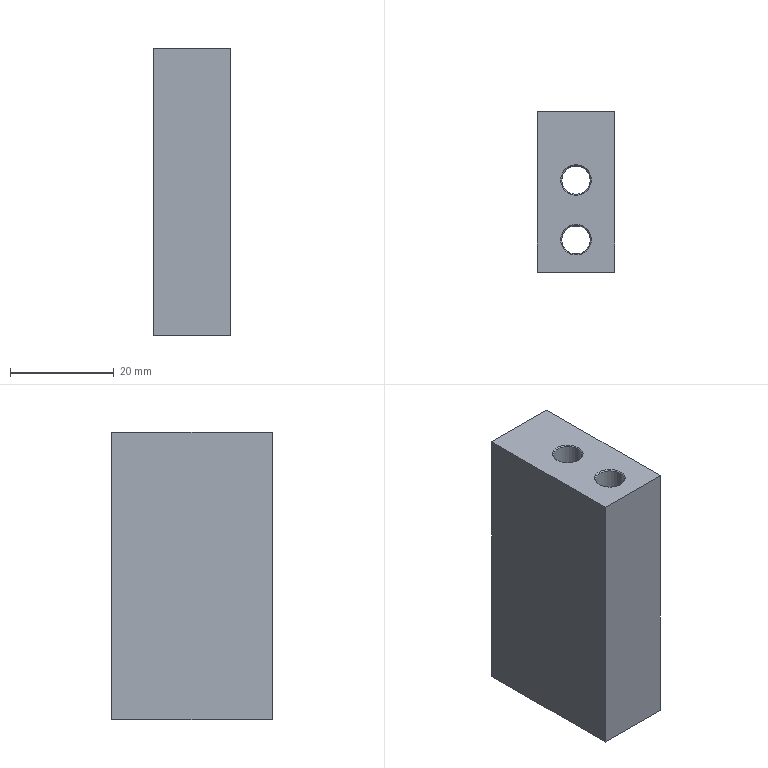Part | NX | 1 solid | 18 faces | box 15 x 31 x 55.4 mm | volume 23127 mm3 | cone 8 | plane 6 | cylinder 4 | commonest cylinder face diameters 5.5 x4
STEP:
#1=CARTESIAN_POINT('',(-70.,176.7,-18.2));
#2=VERTEX_POINT('',#1);
#3=CARTESIAN_POINT('',(-70.,207.7,-18.2));
#4=VERTEX_POINT('',#3);
#5=CARTESIAN_POINT('',(-70.,194.022,-18.2));
#6=DIRECTION('',(0.,1.,0.));
#7=VECTOR('',#6,1000.);
#8=LINE('',#5,#7);
#9=EDGE_CURVE('',#2,#4,#8,.T.);
#10=ORIENTED_EDGE('',*,*,#9,.F.);
#11=CARTESIAN_POINT('',(-70.,176.7,37.2));
#12=VERTEX_POINT('',#11);
#13=CARTESIAN_POINT('',(-70.,176.7,-18.2));
#14=DIRECTION('',(0.,0.,1.));
#15=VECTOR('',#14,1000.);
#16=LINE('',#13,#15);
#17=EDGE_CURVE('',#2,#12,#16,.T.);
#18=ORIENTED_EDGE('',*,*,#17,.T.);
#19=CARTESIAN_POINT('',(-70.,207.7,37.2));
#20=VERTEX_POINT('',#19);
#21=CARTESIAN_POINT('',(-70.,194.022,37.2));
#22=DIRECTION('',(0.,1.,0.));
#23=VECTOR('',#22,1000.);
#24=LINE('',#21,#23);
#25=EDGE_CURVE('',#12,#20,#24,.T.);
#26=ORIENTED_EDGE('',*,*,#25,.T.);
#27=CARTESIAN_POINT('',(-70.,207.7,-18.2));
#28=DIRECTION('',(0.,0.,-1.));
#29=VECTOR('',#28,1000.);
#30=LINE('',#27,#29);
#31=EDGE_CURVE('',#20,#4,#30,.T.);
#32=ORIENTED_EDGE('',*,*,#31,.T.);
#33=EDGE_LOOP('',(#10,#18,#26,#32));
#34=FACE_BOUND('',#33,.T.);
#35=CARTESIAN_POINT('',(-70.,169.7,-18.2));
#36=DIRECTION('',(-1.,0.,0.));
#37=DIRECTION('',(0.,0.,1.));
#38=AXIS2_PLACEMENT_3D('',#35,#36,#37);
#39=PLANE('',#38);
#40=ADVANCED_FACE('',(#34),#39,.T.);
#41=CARTESIAN_POINT('',(-55.,176.7,-18.2));
#42=VERTEX_POINT('',#41);
#43=CARTESIAN_POINT('',(-61.534,176.7,-18.2));
#44=DIRECTION('',(1.,0.,0.));
#45=VECTOR('',#44,1000.);
#46=LINE('',#43,#45);
#47=EDGE_CURVE('',#2,#42,#46,.T.);
#48=ORIENTED_EDGE('',*,*,#47,.T.);
#49=CARTESIAN_POINT('',(-55.,176.7,37.2));
#50=VERTEX_POINT('',#49);
#51=CARTESIAN_POINT('',(-55.,176.7,-18.2));
#52=DIRECTION('',(0.,0.,-1.));
#53=VECTOR('',#52,1000.);
#54=LINE('',#51,#53);
#55=EDGE_CURVE('',#50,#42,#54,.T.);
#56=ORIENTED_EDGE('',*,*,#55,.F.);
#57=CARTESIAN_POINT('',(-61.534,176.7,37.2));
#58=DIRECTION('',(1.,0.,0.));
#59=VECTOR('',#58,1000.);
#60=LINE('',#57,#59);
#61=EDGE_CURVE('',#12,#50,#60,.T.);
#62=ORIENTED_EDGE('',*,*,#61,.F.);
#63=ORIENTED_EDGE('',*,*,#17,.F.);
#64=EDGE_LOOP('',(#48,#56,#62,#63));
#65=FACE_BOUND('',#64,.T.);
#66=CARTESIAN_POINT('',(-55.,176.7,-18.2));
#67=DIRECTION('',(0.,-1.,0.));
#68=DIRECTION('',(0.,0.,-1.));
#69=AXIS2_PLACEMENT_3D('',#66,#67,#68);
#70=PLANE('',#69);
#71=ADVANCED_FACE('',(#65),#70,.T.);
#72=CARTESIAN_POINT('',(-55.,207.7,-18.2));
#73=VERTEX_POINT('',#72);
#74=CARTESIAN_POINT('',(-55.,194.022,-18.2));
#75=DIRECTION('',(0.,-1.,0.));
#76=VECTOR('',#75,1000.);
#77=LINE('',#74,#76);
#78=EDGE_CURVE('',#73,#42,#77,.T.);
#79=ORIENTED_EDGE('',*,*,#78,.F.);
#80=CARTESIAN_POINT('',(-55.,207.7,37.2));
#81=VERTEX_POINT('',#80);
#82=CARTESIAN_POINT('',(-55.,207.7,-18.2));
#83=DIRECTION('',(0.,0.,1.));
#84=VECTOR('',#83,1000.);
#85=LINE('',#82,#84);
#86=EDGE_CURVE('',#73,#81,#85,.T.);
#87=ORIENTED_EDGE('',*,*,#86,.T.);
#88=CARTESIAN_POINT('',(-55.,194.022,37.2));
#89=DIRECTION('',(0.,-1.,0.));
#90=VECTOR('',#89,1000.);
#91=LINE('',#88,#90);
#92=EDGE_CURVE('',#81,#50,#91,.T.);
#93=ORIENTED_EDGE('',*,*,#92,.T.);
#94=ORIENTED_EDGE('',*,*,#55,.T.);
#95=EDGE_LOOP('',(#79,#87,#93,#94));
#96=FACE_BOUND('',#95,.T.);
#97=CARTESIAN_POINT('',(-55.,208.7,-18.2));
#98=DIRECTION('',(1.,0.,0.));
#99=DIRECTION('',(0.,1.,0.));
#100=AXIS2_PLACEMENT_3D('',#97,#98,#99);
#101=PLANE('',#100);
#102=ADVANCED_FACE('',(#96),#101,.T.);
#103=CARTESIAN_POINT('',(-61.534,207.7,-18.2));
#104=DIRECTION('',(-1.,0.,0.));
#105=VECTOR('',#104,1000.);
#106=LINE('',#103,#105);
#107=EDGE_CURVE('',#73,#4,#106,.T.);
#108=ORIENTED_EDGE('',*,*,#107,.T.);
#109=ORIENTED_EDGE('',*,*,#31,.F.);
#110=CARTESIAN_POINT('',(-61.534,207.7,37.2));
#111=DIRECTION('',(-1.,0.,0.));
#112=VECTOR('',#111,1000.);
#113=LINE('',#110,#112);
#114=EDGE_CURVE('',#81,#20,#113,.T.);
#115=ORIENTED_EDGE('',*,*,#114,.F.);
#116=ORIENTED_EDGE('',*,*,#86,.F.);
#117=EDGE_LOOP('',(#108,#109,#115,#116));
#118=FACE_BOUND('',#117,.T.);
#119=CARTESIAN_POINT('',(-70.,207.7,-18.2));
#120=DIRECTION('',(0.,1.,0.));
#121=DIRECTION('',(1.,0.,0.));
#122=AXIS2_PLACEMENT_3D('',#119,#120,#121);
#123=PLANE('',#122);
#124=ADVANCED_FACE('',(#118),#123,.T.);
#125=CARTESIAN_POINT('',(-65.25,194.45,37.));
#126=VERTEX_POINT('',#125);
#127=CARTESIAN_POINT('',(-59.75,194.45,37.));
#128=VERTEX_POINT('',#127);
#129=CARTESIAN_POINT('',(-62.5,194.45,37.));
#130=DIRECTION('',(0.,0.,1.));
#131=DIRECTION('',(1.,0.,0.));
#132=AXIS2_PLACEMENT_3D('',#129,#130,#131);
#133=CIRCLE('',#132,2.75);
#134=EDGE_CURVE('',#126,#128,#133,.T.);
#135=ORIENTED_EDGE('',*,*,#134,.T.);
#136=CARTESIAN_POINT('',(-59.75,194.45,-18.));
#137=VERTEX_POINT('',#136);
#138=CARTESIAN_POINT('',(-59.75,194.45,37.2));
#139=DIRECTION('',(0.,0.,1.));
#140=VECTOR('',#139,1000.);
#141=LINE('',#138,#140);
#142=EDGE_CURVE('',#137,#128,#141,.T.);
#143=ORIENTED_EDGE('',*,*,#142,.F.);
#144=CARTESIAN_POINT('',(-65.25,194.45,-18.));
#145=VERTEX_POINT('',#144);
#146=CARTESIAN_POINT('',(-62.5,194.45,-18.));
#147=DIRECTION('',(0.,0.,1.));
#148=DIRECTION('',(1.,0.,0.));
#149=AXIS2_PLACEMENT_3D('',#146,#147,#148);
#150=CIRCLE('',#149,2.75);
#151=EDGE_CURVE('',#145,#137,#150,.T.);
#152=ORIENTED_EDGE('',*,*,#151,.F.);
#153=CARTESIAN_POINT('',(-65.25,194.45,37.2));
#154=DIRECTION('',(0.,0.,1.));
#155=VECTOR('',#154,1000.);
#156=LINE('',#153,#155);
#157=EDGE_CURVE('',#145,#126,#156,.T.);
#158=ORIENTED_EDGE('',*,*,#157,.T.);
#159=EDGE_LOOP('',(#135,#143,#152,#158));
#160=FACE_BOUND('',#159,.T.);
#161=CARTESIAN_POINT('',(-62.5,194.45,37.2));
#162=DIRECTION('',(0.,0.,1.));
#163=DIRECTION('',(1.,0.,0.));
#164=AXIS2_PLACEMENT_3D('',#161,#162,#163);
#165=CYLINDRICAL_SURFACE('',#164,2.75);
#166=ADVANCED_FACE('',(#160),#165,.F.);
#167=CARTESIAN_POINT('',(-65.45,194.45,37.2));
#168=VERTEX_POINT('',#167);
#169=CARTESIAN_POINT('',(-59.55,194.45,37.2));
#170=VERTEX_POINT('',#169);
#171=CARTESIAN_POINT('',(-62.5,194.45,37.2));
#172=DIRECTION('',(0.,0.,1.));
#173=DIRECTION('',(1.,0.,0.));
#174=AXIS2_PLACEMENT_3D('',#171,#172,#173);
#175=CIRCLE('',#174,2.95);
#176=EDGE_CURVE('',#168,#170,#175,.T.);
#177=ORIENTED_EDGE('',*,*,#176,.T.);
#178=CARTESIAN_POINT('',(-59.75,194.45,37.));
#179=DIRECTION('',(0.7071,0.,0.7071));
#180=VECTOR('',#179,1000.);
#181=LINE('',#178,#180);
#182=EDGE_CURVE('',#128,#170,#181,.T.);
#183=ORIENTED_EDGE('',*,*,#182,.F.);
#184=ORIENTED_EDGE('',*,*,#134,.F.);
#185=CARTESIAN_POINT('',(-65.25,194.45,37.));
#186=DIRECTION('',(-0.7071,0.,0.7071));
#187=VECTOR('',#186,1000.);
#188=LINE('',#185,#187);
#189=EDGE_CURVE('',#126,#168,#188,.T.);
#190=ORIENTED_EDGE('',*,*,#189,.T.);
#191=EDGE_LOOP('',(#177,#183,#184,#190));
#192=FACE_BOUND('',#191,.T.);
#193=CARTESIAN_POINT('',(-62.5,194.45,37.));
#194=DIRECTION('',(0.,0.,1.));
#195=DIRECTION('',(1.,0.,0.));
#196=AXIS2_PLACEMENT_3D('',#193,#194,#195);
#197=CONICAL_SURFACE('',#196,2.75,0.7854);
#198=ADVANCED_FACE('',(#192),#197,.F.);
#199=ORIENTED_EDGE('',*,*,#151,.T.);
#200=CARTESIAN_POINT('',(-59.55,194.45,-18.2));
#201=VERTEX_POINT('',#200);
#202=CARTESIAN_POINT('',(-59.75,194.45,-18.));
#203=DIRECTION('',(0.7071,0.,-0.7071));
#204=VECTOR('',#203,1000.);
#205=LINE('',#202,#204);
#206=EDGE_CURVE('',#201,#137,#205,.F.);
#207=ORIENTED_EDGE('',*,*,#206,.F.);
#208=CARTESIAN_POINT('',(-65.45,194.45,-18.2));
#209=VERTEX_POINT('',#208);
#210=CARTESIAN_POINT('',(-62.5,194.45,-18.2));
#211=DIRECTION('',(0.,0.,1.));
#212=DIRECTION('',(1.,0.,0.));
#213=AXIS2_PLACEMENT_3D('',#210,#211,#212);
#214=CIRCLE('',#213,2.95);
#215=EDGE_CURVE('',#209,#201,#214,.T.);
#216=ORIENTED_EDGE('',*,*,#215,.F.);
#217=CARTESIAN_POINT('',(-65.25,194.45,-18.));
#218=DIRECTION('',(-0.7071,0.,-0.7071));
#219=VECTOR('',#218,1000.);
#220=LINE('',#217,#219);
#221=EDGE_CURVE('',#209,#145,#220,.F.);
#222=ORIENTED_EDGE('',*,*,#221,.T.);
#223=EDGE_LOOP('',(#199,#207,#216,#222));
#224=FACE_BOUND('',#223,.T.);
#225=CARTESIAN_POINT('',(-62.5,194.45,-18.));
#226=DIRECTION('',(0.,0.,-1.));
#227=DIRECTION('',(-1.,0.,0.));
#228=AXIS2_PLACEMENT_3D('',#225,#226,#227);
#229=CONICAL_SURFACE('',#228,2.75,0.7854);
#230=ADVANCED_FACE('',(#224),#229,.F.);
#231=CARTESIAN_POINT('',(-59.75,182.95,-18.));
#232=VERTEX_POINT('',#231);
#233=CARTESIAN_POINT('',(-65.25,182.95,-18.));
#234=VERTEX_POINT('',#233);
#235=CARTESIAN_POINT('',(-62.5,182.95,-18.));
#236=DIRECTION('',(0.,0.,1.));
#237=DIRECTION('',(1.,0.,0.));
#238=AXIS2_PLACEMENT_3D('',#235,#236,#237);
#239=CIRCLE('',#238,2.75);
#240=EDGE_CURVE('',#232,#234,#239,.T.);
#241=ORIENTED_EDGE('',*,*,#240,.T.);
#242=CARTESIAN_POINT('',(-65.45,182.95,-18.2));
#243=VERTEX_POINT('',#242);
#244=CARTESIAN_POINT('',(-65.25,182.95,-18.));
#245=DIRECTION('',(-0.7071,0.,-0.7071));
#246=VECTOR('',#245,1000.);
#247=LINE('',#244,#246);
#248=EDGE_CURVE('',#243,#234,#247,.F.);
#249=ORIENTED_EDGE('',*,*,#248,.F.);
#250=CARTESIAN_POINT('',(-59.55,182.95,-18.2));
#251=VERTEX_POINT('',#250);
#252=CARTESIAN_POINT('',(-62.5,182.95,-18.2));
#253=DIRECTION('',(0.,0.,1.));
#254=DIRECTION('',(1.,0.,0.));
#255=AXIS2_PLACEMENT_3D('',#252,#253,#254);
#256=CIRCLE('',#255,2.95);
#257=EDGE_CURVE('',#251,#243,#256,.T.);
#258=ORIENTED_EDGE('',*,*,#257,.F.);
#259=CARTESIAN_POINT('',(-59.75,182.95,-18.));
#260=DIRECTION('',(0.7071,0.,-0.7071));
#261=VECTOR('',#260,1000.);
#262=LINE('',#259,#261);
#263=EDGE_CURVE('',#251,#232,#262,.F.);
#264=ORIENTED_EDGE('',*,*,#263,.T.);
#265=EDGE_LOOP('',(#241,#249,#258,#264));
#266=FACE_BOUND('',#265,.T.);
#267=CARTESIAN_POINT('',(-62.5,182.95,-18.));
#268=DIRECTION('',(0.,0.,-1.));
#269=DIRECTION('',(-1.,0.,0.));
#270=AXIS2_PLACEMENT_3D('',#267,#268,#269);
#271=CONICAL_SURFACE('',#270,2.75,0.7854);
#272=ADVANCED_FACE('',(#266),#271,.F.);
#273=CARTESIAN_POINT('',(-65.25,182.95,37.));
#274=VERTEX_POINT('',#273);
#275=CARTESIAN_POINT('',(-59.75,182.95,37.));
#276=VERTEX_POINT('',#275);
#277=CARTESIAN_POINT('',(-62.5,182.95,37.));
#278=DIRECTION('',(0.,0.,1.));
#279=DIRECTION('',(1.,0.,0.));
#280=AXIS2_PLACEMENT_3D('',#277,#278,#279);
#281=CIRCLE('',#280,2.75);
#282=EDGE_CURVE('',#274,#276,#281,.T.);
#283=ORIENTED_EDGE('',*,*,#282,.F.);
#284=CARTESIAN_POINT('',(-65.45,182.95,37.2));
#285=VERTEX_POINT('',#284);
#286=CARTESIAN_POINT('',(-65.25,182.95,37.));
#287=DIRECTION('',(-0.7071,0.,0.7071));
#288=VECTOR('',#287,1000.);
#289=LINE('',#286,#288);
#290=EDGE_CURVE('',#285,#274,#289,.F.);
#291=ORIENTED_EDGE('',*,*,#290,.F.);
#292=CARTESIAN_POINT('',(-59.55,182.95,37.2));
#293=VERTEX_POINT('',#292);
#294=CARTESIAN_POINT('',(-62.5,182.95,37.2));
#295=DIRECTION('',(0.,0.,1.));
#296=DIRECTION('',(1.,0.,0.));
#297=AXIS2_PLACEMENT_3D('',#294,#295,#296);
#298=CIRCLE('',#297,2.95);
#299=EDGE_CURVE('',#285,#293,#298,.T.);
#300=ORIENTED_EDGE('',*,*,#299,.T.);
#301=CARTESIAN_POINT('',(-59.75,182.95,37.));
#302=DIRECTION('',(0.7071,0.,0.7071));
#303=VECTOR('',#302,1000.);
#304=LINE('',#301,#303);
#305=EDGE_CURVE('',#293,#276,#304,.F.);
#306=ORIENTED_EDGE('',*,*,#305,.T.);
#307=EDGE_LOOP('',(#283,#291,#300,#306));
#308=FACE_BOUND('',#307,.T.);
#309=CARTESIAN_POINT('',(-62.5,182.95,37.));
#310=DIRECTION('',(0.,0.,1.));
#311=DIRECTION('',(1.,0.,0.));
#312=AXIS2_PLACEMENT_3D('',#309,#310,#311);
#313=CONICAL_SURFACE('',#312,2.75,0.7854);
#314=ADVANCED_FACE('',(#308),#313,.F.);
#315=ORIENTED_EDGE('',*,*,#47,.F.);
#316=ORIENTED_EDGE('',*,*,#9,.T.);
#317=ORIENTED_EDGE('',*,*,#107,.F.);
#318=ORIENTED_EDGE('',*,*,#78,.T.);
#319=EDGE_LOOP('',(#315,#316,#317,#318));
#320=FACE_BOUND('',#319,.T.);
#321=ORIENTED_EDGE('',*,*,#215,.T.);
#322=CARTESIAN_POINT('',(-62.5,194.45,-18.2));
#323=DIRECTION('',(0.,0.,1.));
#324=DIRECTION('',(1.,0.,0.));
#325=AXIS2_PLACEMENT_3D('',#322,#323,#324);
#326=CIRCLE('',#325,2.95);
#327=EDGE_CURVE('',#201,#209,#326,.T.);
#328=ORIENTED_EDGE('',*,*,#327,.T.);
#329=EDGE_LOOP('',(#321,#328));
#330=FACE_BOUND('',#329,.T.);
#331=CARTESIAN_POINT('',(-62.5,182.95,-18.2));
#332=DIRECTION('',(0.,0.,1.));
#333=DIRECTION('',(1.,0.,0.));
#334=AXIS2_PLACEMENT_3D('',#331,#332,#333);
#335=CIRCLE('',#334,2.95);
#336=EDGE_CURVE('',#243,#251,#335,.T.);
#337=ORIENTED_EDGE('',*,*,#336,.T.);
#338=ORIENTED_EDGE('',*,*,#257,.T.);
#339=EDGE_LOOP('',(#337,#338));
#340=FACE_BOUND('',#339,.T.);
#341=CARTESIAN_POINT('',(-61.534,194.022,-18.2));
#342=DIRECTION('',(0.,0.,1.));
#343=DIRECTION('',(1.,0.,0.));
#344=AXIS2_PLACEMENT_3D('',#341,#342,#343);
#345=PLANE('',#344);
#346=ADVANCED_FACE('',(#320,#330,#340),#345,.F.);
#347=ORIENTED_EDGE('',*,*,#92,.F.);
#348=ORIENTED_EDGE('',*,*,#114,.T.);
#349=ORIENTED_EDGE('',*,*,#25,.F.);
#350=ORIENTED_EDGE('',*,*,#61,.T.);
#351=EDGE_LOOP('',(#347,#348,#349,#350));
#352=FACE_BOUND('',#351,.T.);
#353=ORIENTED_EDGE('',*,*,#176,.F.);
#354=CARTESIAN_POINT('',(-62.5,194.45,37.2));
#355=DIRECTION('',(0.,0.,1.));
#356=DIRECTION('',(1.,0.,0.));
#357=AXIS2_PLACEMENT_3D('',#354,#355,#356);
#358=CIRCLE('',#357,2.95);
#359=EDGE_CURVE('',#170,#168,#358,.T.);
#360=ORIENTED_EDGE('',*,*,#359,.F.);
#361=EDGE_LOOP('',(#353,#360));
#362=FACE_BOUND('',#361,.T.);
#363=CARTESIAN_POINT('',(-62.5,182.95,37.2));
#364=DIRECTION('',(0.,0.,1.));
#365=DIRECTION('',(1.,0.,0.));
#366=AXIS2_PLACEMENT_3D('',#363,#364,#365);
#367=CIRCLE('',#366,2.95);
#368=EDGE_CURVE('',#293,#285,#367,.T.);
#369=ORIENTED_EDGE('',*,*,#368,.F.);
#370=ORIENTED_EDGE('',*,*,#299,.F.);
#371=EDGE_LOOP('',(#369,#370));
#372=FACE_BOUND('',#371,.T.);
#373=CARTESIAN_POINT('',(-61.534,194.022,37.2));
#374=DIRECTION('',(0.,0.,1.));
#375=DIRECTION('',(1.,0.,0.));
#376=AXIS2_PLACEMENT_3D('',#373,#374,#375);
#377=PLANE('',#376);
#378=ADVANCED_FACE('',(#352,#362,#372),#377,.T.);
#379=ORIENTED_EDGE('',*,*,#240,.F.);
#380=CARTESIAN_POINT('',(-59.75,182.95,37.2));
#381=DIRECTION('',(0.,0.,1.));
#382=VECTOR('',#381,1000.);
#383=LINE('',#380,#382);
#384=EDGE_CURVE('',#232,#276,#383,.T.);
#385=ORIENTED_EDGE('',*,*,#384,.T.);
#386=CARTESIAN_POINT('',(-62.5,182.95,37.));
#387=DIRECTION('',(0.,0.,1.));
#388=DIRECTION('',(1.,0.,0.));
#389=AXIS2_PLACEMENT_3D('',#386,#387,#388);
#390=CIRCLE('',#389,2.75);
#391=EDGE_CURVE('',#276,#274,#390,.T.);
#392=ORIENTED_EDGE('',*,*,#391,.T.);
#393=CARTESIAN_POINT('',(-65.25,182.95,37.2));
#394=DIRECTION('',(0.,0.,1.));
#395=VECTOR('',#394,1000.);
#396=LINE('',#393,#395);
#397=EDGE_CURVE('',#234,#274,#396,.T.);
#398=ORIENTED_EDGE('',*,*,#397,.F.);
#399=EDGE_LOOP('',(#379,#385,#392,#398));
#400=FACE_BOUND('',#399,.T.);
#401=CARTESIAN_POINT('',(-62.5,182.95,37.2));
#402=DIRECTION('',(0.,0.,1.));
#403=DIRECTION('',(1.,0.,0.));
#404=AXIS2_PLACEMENT_3D('',#401,#402,#403);
#405=CYLINDRICAL_SURFACE('',#404,2.75);
#406=ADVANCED_FACE('',(#400),#405,.F.);
#407=ORIENTED_EDGE('',*,*,#368,.T.);
#408=ORIENTED_EDGE('',*,*,#290,.T.);
#409=ORIENTED_EDGE('',*,*,#391,.F.);
#410=ORIENTED_EDGE('',*,*,#305,.F.);
#411=EDGE_LOOP('',(#407,#408,#409,#410));
#412=FACE_BOUND('',#411,.T.);
#413=CARTESIAN_POINT('',(-62.5,182.95,37.));
#414=DIRECTION('',(0.,0.,1.));
#415=DIRECTION('',(1.,0.,0.));
#416=AXIS2_PLACEMENT_3D('',#413,#414,#415);
#417=CONICAL_SURFACE('',#416,2.75,0.7854);
#418=ADVANCED_FACE('',(#412),#417,.F.);
#419=ORIENTED_EDGE('',*,*,#182,.T.);
#420=ORIENTED_EDGE('',*,*,#359,.T.);
#421=ORIENTED_EDGE('',*,*,#189,.F.);
#422=CARTESIAN_POINT('',(-62.5,194.45,37.));
#423=DIRECTION('',(0.,0.,1.));
#424=DIRECTION('',(1.,0.,0.));
#425=AXIS2_PLACEMENT_3D('',#422,#423,#424);
#426=CIRCLE('',#425,2.75);
#427=EDGE_CURVE('',#128,#126,#426,.T.);
#428=ORIENTED_EDGE('',*,*,#427,.F.);
#429=EDGE_LOOP('',(#419,#420,#421,#428));
#430=FACE_BOUND('',#429,.T.);
#431=CARTESIAN_POINT('',(-62.5,194.45,37.));
#432=DIRECTION('',(0.,0.,1.));
#433=DIRECTION('',(1.,0.,0.));
#434=AXIS2_PLACEMENT_3D('',#431,#432,#433);
#435=CONICAL_SURFACE('',#434,2.75,0.7854);
#436=ADVANCED_FACE('',(#430),#435,.F.);
#437=ORIENTED_EDGE('',*,*,#142,.T.);
#438=ORIENTED_EDGE('',*,*,#427,.T.);
#439=ORIENTED_EDGE('',*,*,#157,.F.);
#440=CARTESIAN_POINT('',(-62.5,194.45,-18.));
#441=DIRECTION('',(0.,0.,1.));
#442=DIRECTION('',(1.,0.,0.));
#443=AXIS2_PLACEMENT_3D('',#440,#441,#442);
#444=CIRCLE('',#443,2.75);
#445=EDGE_CURVE('',#137,#145,#444,.T.);
#446=ORIENTED_EDGE('',*,*,#445,.F.);
#447=EDGE_LOOP('',(#437,#438,#439,#446));
#448=FACE_BOUND('',#447,.T.);
#449=CARTESIAN_POINT('',(-62.5,194.45,37.2));
#450=DIRECTION('',(0.,0.,1.));
#451=DIRECTION('',(1.,0.,0.));
#452=AXIS2_PLACEMENT_3D('',#449,#450,#451);
#453=CYLINDRICAL_SURFACE('',#452,2.75);
#454=ADVANCED_FACE('',(#448),#453,.F.);
#455=ORIENTED_EDGE('',*,*,#221,.F.);
#456=ORIENTED_EDGE('',*,*,#327,.F.);
#457=ORIENTED_EDGE('',*,*,#206,.T.);
#458=ORIENTED_EDGE('',*,*,#445,.T.);
#459=EDGE_LOOP('',(#455,#456,#457,#458));
#460=FACE_BOUND('',#459,.T.);
#461=CARTESIAN_POINT('',(-62.5,194.45,-18.));
#462=DIRECTION('',(0.,0.,-1.));
#463=DIRECTION('',(-1.,0.,0.));
#464=AXIS2_PLACEMENT_3D('',#461,#462,#463);
#465=CONICAL_SURFACE('',#464,2.75,0.7854);
#466=ADVANCED_FACE('',(#460),#465,.F.);
#467=ORIENTED_EDGE('',*,*,#336,.F.);
#468=ORIENTED_EDGE('',*,*,#248,.T.);
#469=CARTESIAN_POINT('',(-62.5,182.95,-18.));
#470=DIRECTION('',(0.,0.,1.));
#471=DIRECTION('',(1.,0.,0.));
#472=AXIS2_PLACEMENT_3D('',#469,#470,#471);
#473=CIRCLE('',#472,2.75);
#474=EDGE_CURVE('',#234,#232,#473,.T.);
#475=ORIENTED_EDGE('',*,*,#474,.T.);
#476=ORIENTED_EDGE('',*,*,#263,.F.);
#477=EDGE_LOOP('',(#467,#468,#475,#476));
#478=FACE_BOUND('',#477,.T.);
#479=CARTESIAN_POINT('',(-62.5,182.95,-18.));
#480=DIRECTION('',(0.,0.,-1.));
#481=DIRECTION('',(-1.,0.,0.));
#482=AXIS2_PLACEMENT_3D('',#479,#480,#481);
#483=CONICAL_SURFACE('',#482,2.75,0.7854);
#484=ADVANCED_FACE('',(#478),#483,.F.);
#485=ORIENTED_EDGE('',*,*,#282,.T.);
#486=ORIENTED_EDGE('',*,*,#384,.F.);
#487=ORIENTED_EDGE('',*,*,#474,.F.);
#488=ORIENTED_EDGE('',*,*,#397,.T.);
#489=EDGE_LOOP('',(#485,#486,#487,#488));
#490=FACE_BOUND('',#489,.T.);
#491=CARTESIAN_POINT('',(-62.5,182.95,37.2));
#492=DIRECTION('',(0.,0.,1.));
#493=DIRECTION('',(1.,0.,0.));
#494=AXIS2_PLACEMENT_3D('',#491,#492,#493);
#495=CYLINDRICAL_SURFACE('',#494,2.75);
#496=ADVANCED_FACE('',(#490),#495,.F.);
#497=CLOSED_SHELL('',(#40,#71,#102,#124,#166,#198,#230,#272,#314,#346,#378,#406,#418,#436,#454,#466,#484,#496));
#498=MANIFOLD_SOLID_BREP('',#497);
#499=(LENGTH_UNIT()NAMED_UNIT(*)SI_UNIT(.MILLI.,.METRE.));
#500=UNCERTAINTY_MEASURE_WITH_UNIT(LENGTH_MEASURE(0.00001),#499,'','');
#501=(NAMED_UNIT(*)PLANE_ANGLE_UNIT()SI_UNIT($,.RADIAN.));
#502=(NAMED_UNIT(*)SI_UNIT($,.STERADIAN.)SOLID_ANGLE_UNIT());
#503=(GEOMETRIC_REPRESENTATION_CONTEXT(3)GLOBAL_UNCERTAINTY_ASSIGNED_CONTEXT((#500))GLOBAL_UNIT_ASSIGNED_CONTEXT((#499,#501,#502))REPRESENTATION_CONTEXT('',''));
#504=ADVANCED_BREP_SHAPE_REPRESENTATION('',(#498),#503);